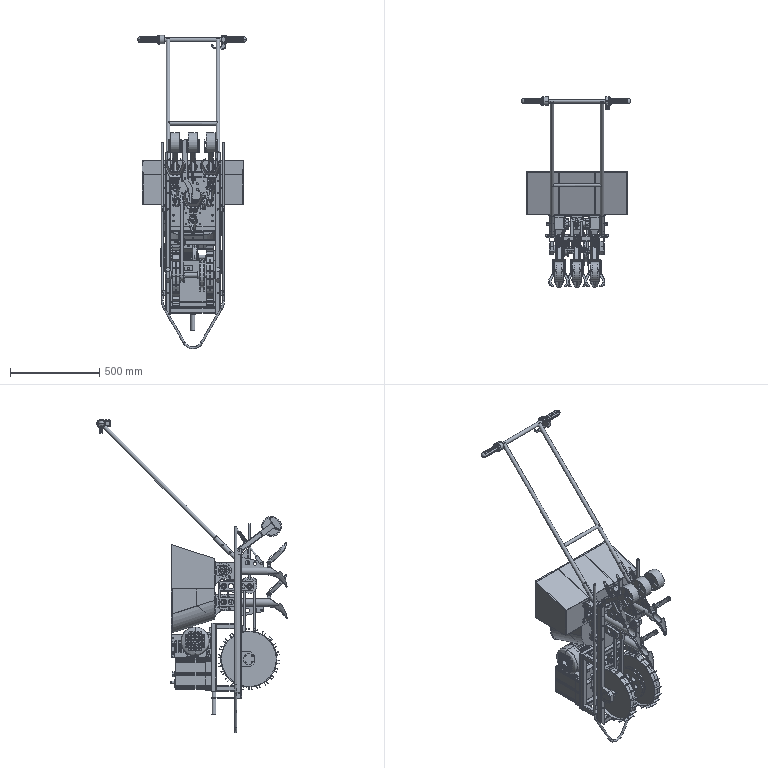Part | NX | features EXTRUDE 114, DATUM_CSYS 75, SKETCH 74, EXTRACT_DATUM_PLANE 45, BREP 36, EXTRACT_BODY 25, UNITE 18, LINKED_FACE 16, BLEND 10, LINKED_BODY 5, SHELL 5, CHAMFER 4, SUBTRACT 4, SWP104 4, INTERSECT 3, DATUM_PLANE 2, Delete Body 2, EXTRACT_STRING 2, Pattern Geometry 2, Container 1, DRAFT 1, Geometry Instance 1, HOLE PACKAGE 1, Instance Feature 1, MOVE_FACE 1, Mirror Feature 1, OFFSET 1, REPLACE_FACE 1, SCALE 1, SIMPLE HOLE 1, SYMBOLIC_THREAD 1 | 250 solids | 6867 faces | volume 25576311 mm3 | plane 3440 | cylinder 2562 | torus 381 | cone 230 | spline 152 | sphere 102 | commonest cylinder face diameters 2 x187 10 x167 8 x152 4.8 x102 7.77 x99 30 x92